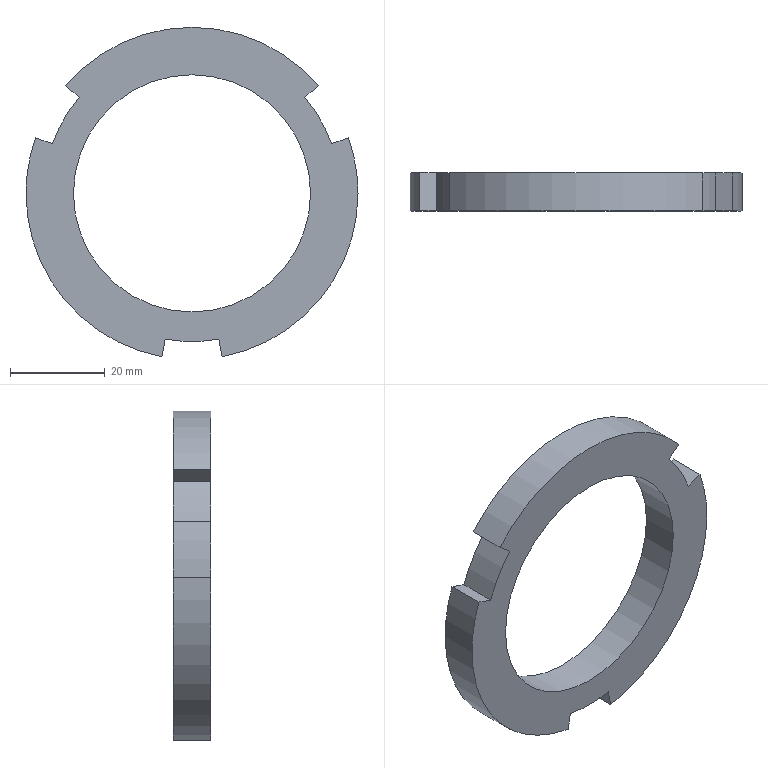Part | STEP file | Input 1-6 | 1 solid | 18 faces | box 70 x 8 x 69.422 mm | volume 13993 mm3 | cylinder 10 | plane 8 | commonest cylinder face diameters 70 x5 62.489 x3 50 x2
STEP:
#1=CARTESIAN_POINT('',(-583.859,1957.264,3172.342));
#2=VERTEX_POINT('',#1);
#3=CARTESIAN_POINT('',(-612.523,1957.264,3137.92));
#4=VERTEX_POINT('',#3);
#5=CARTESIAN_POINT('',(-618.859,1957.264,3172.342));
#6=DIRECTION('',(0.,1.,0.));
#7=DIRECTION('',(1.,0.,0.));
#8=AXIS2_PLACEMENT_3D('',#5,#6,#7);
#9=CIRCLE('',#8,35.);
#10=EDGE_CURVE('',#2,#4,#9,.T.);
#11=ORIENTED_EDGE('',*,*,#10,.F.);
#12=CARTESIAN_POINT('',(-583.859,1949.264,3172.342));
#13=VERTEX_POINT('',#12);
#14=CARTESIAN_POINT('',(-583.859,1957.264,3172.342));
#15=DIRECTION('',(0.,-1.,0.));
#16=VECTOR('',#15,1000.);
#17=LINE('',#14,#16);
#18=EDGE_CURVE('',#2,#13,#17,.T.);
#19=ORIENTED_EDGE('',*,*,#18,.T.);
#20=CARTESIAN_POINT('',(-612.523,1949.264,3137.92));
#21=VERTEX_POINT('',#20);
#22=CARTESIAN_POINT('',(-618.859,1949.264,3172.342));
#23=DIRECTION('',(0.,1.,0.));
#24=DIRECTION('',(1.,0.,0.));
#25=AXIS2_PLACEMENT_3D('',#22,#23,#24);
#26=CIRCLE('',#25,35.);
#27=EDGE_CURVE('',#13,#21,#26,.T.);
#28=ORIENTED_EDGE('',*,*,#27,.T.);
#29=CARTESIAN_POINT('',(-612.523,1957.264,3137.92));
#30=DIRECTION('',(0.,-1.,0.));
#31=VECTOR('',#30,1000.);
#32=LINE('',#29,#31);
#33=EDGE_CURVE('',#4,#21,#32,.T.);
#34=ORIENTED_EDGE('',*,*,#33,.F.);
#35=EDGE_LOOP('',(#11,#19,#28,#34));
#36=FACE_OUTER_BOUND('',#35,.T.);
#37=CARTESIAN_POINT('',(-618.859,1957.264,3172.342));
#38=DIRECTION('',(0.,-1.,0.));
#39=DIRECTION('',(1.,0.,0.));
#40=AXIS2_PLACEMENT_3D('',#37,#38,#39);
#41=CYLINDRICAL_SURFACE('',#40,35.);
#42=ADVANCED_FACE('',(#36),#41,.T.);
#43=CARTESIAN_POINT('',(-643.859,1957.264,3172.342));
#44=VERTEX_POINT('',#43);
#45=CARTESIAN_POINT('',(-593.859,1957.264,3172.342));
#46=VERTEX_POINT('',#45);
#47=CARTESIAN_POINT('',(-618.859,1957.264,3172.342));
#48=DIRECTION('',(0.,1.,0.));
#49=DIRECTION('',(1.,0.,0.));
#50=AXIS2_PLACEMENT_3D('',#47,#48,#49);
#51=CIRCLE('',#50,25.);
#52=EDGE_CURVE('',#44,#46,#51,.T.);
#53=ORIENTED_EDGE('',*,*,#52,.T.);
#54=CARTESIAN_POINT('',(-593.859,1949.264,3172.342));
#55=VERTEX_POINT('',#54);
#56=CARTESIAN_POINT('',(-593.859,1957.264,3172.342));
#57=DIRECTION('',(0.,1.,0.));
#58=VECTOR('',#57,1000.);
#59=LINE('',#56,#58);
#60=EDGE_CURVE('',#55,#46,#59,.T.);
#61=ORIENTED_EDGE('',*,*,#60,.F.);
#62=CARTESIAN_POINT('',(-643.859,1949.264,3172.342));
#63=VERTEX_POINT('',#62);
#64=CARTESIAN_POINT('',(-618.859,1949.264,3172.342));
#65=DIRECTION('',(0.,1.,0.));
#66=DIRECTION('',(1.,0.,0.));
#67=AXIS2_PLACEMENT_3D('',#64,#65,#66);
#68=CIRCLE('',#67,25.);
#69=EDGE_CURVE('',#63,#55,#68,.T.);
#70=ORIENTED_EDGE('',*,*,#69,.F.);
#71=CARTESIAN_POINT('',(-643.859,1957.264,3172.342));
#72=DIRECTION('',(0.,1.,0.));
#73=VECTOR('',#72,1000.);
#74=LINE('',#71,#73);
#75=EDGE_CURVE('',#63,#44,#74,.T.);
#76=ORIENTED_EDGE('',*,*,#75,.T.);
#77=EDGE_LOOP('',(#53,#61,#70,#76));
#78=FACE_OUTER_BOUND('',#77,.T.);
#79=CARTESIAN_POINT('',(-618.859,1957.264,3172.342));
#80=DIRECTION('',(0.,-1.,0.));
#81=DIRECTION('',(1.,0.,0.));
#82=AXIS2_PLACEMENT_3D('',#79,#80,#81);
#83=CYLINDRICAL_SURFACE('',#82,25.);
#84=ADVANCED_FACE('',(#78),#83,.F.);
#85=CARTESIAN_POINT('',(-653.859,1957.264,3172.342));
#86=VERTEX_POINT('',#85);
#87=CARTESIAN_POINT('',(-651.837,1957.264,3184.066));
#88=VERTEX_POINT('',#87);
#89=CARTESIAN_POINT('',(-618.859,1957.264,3172.342));
#90=DIRECTION('',(0.,1.,0.));
#91=DIRECTION('',(1.,0.,0.));
#92=AXIS2_PLACEMENT_3D('',#89,#90,#91);
#93=CIRCLE('',#92,35.);
#94=EDGE_CURVE('',#86,#88,#93,.T.);
#95=ORIENTED_EDGE('',*,*,#94,.F.);
#96=CARTESIAN_POINT('',(-653.859,1949.264,3172.342));
#97=VERTEX_POINT('',#96);
#98=CARTESIAN_POINT('',(-653.859,1957.264,3172.342));
#99=DIRECTION('',(0.,-1.,0.));
#100=VECTOR('',#99,1000.);
#101=LINE('',#98,#100);
#102=EDGE_CURVE('',#86,#97,#101,.T.);
#103=ORIENTED_EDGE('',*,*,#102,.T.);
#104=CARTESIAN_POINT('',(-651.837,1949.264,3184.066));
#105=VERTEX_POINT('',#104);
#106=CARTESIAN_POINT('',(-618.859,1949.264,3172.342));
#107=DIRECTION('',(0.,1.,0.));
#108=DIRECTION('',(1.,0.,0.));
#109=AXIS2_PLACEMENT_3D('',#106,#107,#108);
#110=CIRCLE('',#109,35.);
#111=EDGE_CURVE('',#97,#105,#110,.T.);
#112=ORIENTED_EDGE('',*,*,#111,.T.);
#113=CARTESIAN_POINT('',(-651.837,1957.264,3184.066));
#114=DIRECTION('',(0.,-1.,0.));
#115=VECTOR('',#114,1000.);
#116=LINE('',#113,#115);
#117=EDGE_CURVE('',#88,#105,#116,.T.);
#118=ORIENTED_EDGE('',*,*,#117,.F.);
#119=EDGE_LOOP('',(#95,#103,#112,#118));
#120=FACE_OUTER_BOUND('',#119,.T.);
#121=CARTESIAN_POINT('',(-618.859,1957.264,3172.342));
#122=DIRECTION('',(0.,-1.,0.));
#123=DIRECTION('',(1.,0.,0.));
#124=AXIS2_PLACEMENT_3D('',#121,#122,#123);
#125=CYLINDRICAL_SURFACE('',#124,35.);
#126=ADVANCED_FACE('',(#120),#125,.T.);
#127=CARTESIAN_POINT('',(-613.203,1957.264,3141.613));
#128=VERTEX_POINT('',#127);
#129=CARTESIAN_POINT('',(-624.515,1957.264,3141.613));
#130=VERTEX_POINT('',#129);
#131=CARTESIAN_POINT('',(-618.859,1957.264,3172.342));
#132=DIRECTION('',(0.,1.,0.));
#133=DIRECTION('',(1.,0.,0.));
#134=AXIS2_PLACEMENT_3D('',#131,#132,#133);
#135=CIRCLE('',#134,31.244);
#136=EDGE_CURVE('',#128,#130,#135,.T.);
#137=ORIENTED_EDGE('',*,*,#136,.T.);
#138=CARTESIAN_POINT('',(-625.195,1957.264,3137.92));
#139=VERTEX_POINT('',#138);
#140=CARTESIAN_POINT('',(-625.195,1957.264,3137.92));
#141=DIRECTION('',(-0.181,0.,-0.9835));
#142=VECTOR('',#141,1000.);
#143=LINE('',#140,#142);
#144=EDGE_CURVE('',#130,#139,#143,.T.);
#145=ORIENTED_EDGE('',*,*,#144,.T.);
#146=CARTESIAN_POINT('',(-618.859,1957.264,3172.342));
#147=DIRECTION('',(0.,1.,0.));
#148=DIRECTION('',(1.,0.,0.));
#149=AXIS2_PLACEMENT_3D('',#146,#147,#148);
#150=CIRCLE('',#149,35.);
#151=EDGE_CURVE('',#139,#86,#150,.T.);
#152=ORIENTED_EDGE('',*,*,#151,.T.);
#153=ORIENTED_EDGE('',*,*,#94,.T.);
#154=CARTESIAN_POINT('',(-648.298,1957.264,3182.808));
#155=VERTEX_POINT('',#154);
#156=CARTESIAN_POINT('',(-651.837,1957.264,3184.066));
#157=DIRECTION('',(0.9422,0.,-0.335));
#158=VECTOR('',#157,1000.);
#159=LINE('',#156,#158);
#160=EDGE_CURVE('',#88,#155,#159,.T.);
#161=ORIENTED_EDGE('',*,*,#160,.T.);
#162=CARTESIAN_POINT('',(-642.642,1957.264,3192.604));
#163=VERTEX_POINT('',#162);
#164=CARTESIAN_POINT('',(-618.859,1957.264,3172.342));
#165=DIRECTION('',(0.,1.,0.));
#166=DIRECTION('',(1.,0.,0.));
#167=AXIS2_PLACEMENT_3D('',#164,#165,#166);
#168=CIRCLE('',#167,31.244);
#169=EDGE_CURVE('',#155,#163,#168,.T.);
#170=ORIENTED_EDGE('',*,*,#169,.T.);
#171=CARTESIAN_POINT('',(-645.501,1957.264,3195.04));
#172=VERTEX_POINT('',#171);
#173=CARTESIAN_POINT('',(-645.501,1957.264,3195.04));
#174=DIRECTION('',(-0.7612,0.,0.6485));
#175=VECTOR('',#174,1000.);
#176=LINE('',#173,#175);
#177=EDGE_CURVE('',#163,#172,#176,.T.);
#178=ORIENTED_EDGE('',*,*,#177,.T.);
#179=CARTESIAN_POINT('',(-592.217,1957.264,3195.04));
#180=VERTEX_POINT('',#179);
#181=CARTESIAN_POINT('',(-618.859,1957.264,3172.342));
#182=DIRECTION('',(0.,1.,0.));
#183=DIRECTION('',(1.,0.,0.));
#184=AXIS2_PLACEMENT_3D('',#181,#182,#183);
#185=CIRCLE('',#184,35.);
#186=EDGE_CURVE('',#172,#180,#185,.T.);
#187=ORIENTED_EDGE('',*,*,#186,.T.);
#188=CARTESIAN_POINT('',(-595.075,1957.264,3192.604));
#189=VERTEX_POINT('',#188);
#190=CARTESIAN_POINT('',(-592.217,1957.264,3195.04));
#191=DIRECTION('',(-0.7612,0.,-0.6485));
#192=VECTOR('',#191,1000.);
#193=LINE('',#190,#192);
#194=EDGE_CURVE('',#180,#189,#193,.T.);
#195=ORIENTED_EDGE('',*,*,#194,.T.);
#196=CARTESIAN_POINT('',(-589.419,1957.264,3182.808));
#197=VERTEX_POINT('',#196);
#198=CARTESIAN_POINT('',(-618.859,1957.264,3172.342));
#199=DIRECTION('',(0.,1.,0.));
#200=DIRECTION('',(1.,0.,0.));
#201=AXIS2_PLACEMENT_3D('',#198,#199,#200);
#202=CIRCLE('',#201,31.244);
#203=EDGE_CURVE('',#189,#197,#202,.T.);
#204=ORIENTED_EDGE('',*,*,#203,.T.);
#205=CARTESIAN_POINT('',(-585.881,1957.264,3184.066));
#206=VERTEX_POINT('',#205);
#207=CARTESIAN_POINT('',(-585.881,1957.264,3184.066));
#208=DIRECTION('',(0.9422,0.,0.335));
#209=VECTOR('',#208,1000.);
#210=LINE('',#207,#209);
#211=EDGE_CURVE('',#197,#206,#210,.T.);
#212=ORIENTED_EDGE('',*,*,#211,.T.);
#213=CARTESIAN_POINT('',(-618.859,1957.264,3172.342));
#214=DIRECTION('',(0.,1.,0.));
#215=DIRECTION('',(1.,0.,0.));
#216=AXIS2_PLACEMENT_3D('',#213,#214,#215);
#217=CIRCLE('',#216,35.);
#218=EDGE_CURVE('',#206,#2,#217,.T.);
#219=ORIENTED_EDGE('',*,*,#218,.T.);
#220=ORIENTED_EDGE('',*,*,#10,.T.);
#221=CARTESIAN_POINT('',(-612.523,1957.264,3137.92));
#222=DIRECTION('',(-0.181,0.,0.9835));
#223=VECTOR('',#222,1000.);
#224=LINE('',#221,#223);
#225=EDGE_CURVE('',#4,#128,#224,.T.);
#226=ORIENTED_EDGE('',*,*,#225,.T.);
#227=EDGE_LOOP('',(#137,#145,#152,#153,#161,#170,#178,#187,#195,#204,#212,#219,#220,#226));
#228=FACE_OUTER_BOUND('',#227,.T.);
#229=ORIENTED_EDGE('',*,*,#52,.F.);
#230=CARTESIAN_POINT('',(-618.859,1957.264,3172.342));
#231=DIRECTION('',(0.,1.,0.));
#232=DIRECTION('',(1.,0.,0.));
#233=AXIS2_PLACEMENT_3D('',#230,#231,#232);
#234=CIRCLE('',#233,25.);
#235=EDGE_CURVE('',#46,#44,#234,.T.);
#236=ORIENTED_EDGE('',*,*,#235,.F.);
#237=EDGE_LOOP('',(#229,#236));
#238=FACE_BOUND('',#237,.T.);
#239=CARTESIAN_POINT('',(-618.859,1957.264,3172.342));
#240=DIRECTION('',(0.,1.,0.));
#241=DIRECTION('',(-1.,0.,0.));
#242=AXIS2_PLACEMENT_3D('',#239,#240,#241);
#243=PLANE('',#242);
#244=ADVANCED_FACE('',(#228,#238),#243,.T.);
#245=CARTESIAN_POINT('',(-613.203,1949.264,3141.613));
#246=VERTEX_POINT('',#245);
#247=CARTESIAN_POINT('',(-624.515,1949.264,3141.613));
#248=VERTEX_POINT('',#247);
#249=CARTESIAN_POINT('',(-618.859,1949.264,3172.342));
#250=DIRECTION('',(0.,1.,0.));
#251=DIRECTION('',(1.,0.,0.));
#252=AXIS2_PLACEMENT_3D('',#249,#250,#251);
#253=CIRCLE('',#252,31.244);
#254=EDGE_CURVE('',#246,#248,#253,.T.);
#255=ORIENTED_EDGE('',*,*,#254,.F.);
#256=CARTESIAN_POINT('',(-612.523,1949.264,3137.92));
#257=DIRECTION('',(-0.181,0.,0.9835));
#258=VECTOR('',#257,1000.);
#259=LINE('',#256,#258);
#260=EDGE_CURVE('',#21,#246,#259,.T.);
#261=ORIENTED_EDGE('',*,*,#260,.F.);
#262=ORIENTED_EDGE('',*,*,#27,.F.);
#263=CARTESIAN_POINT('',(-585.881,1949.264,3184.066));
#264=VERTEX_POINT('',#263);
#265=CARTESIAN_POINT('',(-618.859,1949.264,3172.342));
#266=DIRECTION('',(0.,1.,0.));
#267=DIRECTION('',(1.,0.,0.));
#268=AXIS2_PLACEMENT_3D('',#265,#266,#267);
#269=CIRCLE('',#268,35.);
#270=EDGE_CURVE('',#264,#13,#269,.T.);
#271=ORIENTED_EDGE('',*,*,#270,.F.);
#272=CARTESIAN_POINT('',(-589.419,1949.264,3182.808));
#273=VERTEX_POINT('',#272);
#274=CARTESIAN_POINT('',(-585.881,1949.264,3184.066));
#275=DIRECTION('',(0.9422,0.,0.335));
#276=VECTOR('',#275,1000.);
#277=LINE('',#274,#276);
#278=EDGE_CURVE('',#273,#264,#277,.T.);
#279=ORIENTED_EDGE('',*,*,#278,.F.);
#280=CARTESIAN_POINT('',(-595.075,1949.264,3192.604));
#281=VERTEX_POINT('',#280);
#282=CARTESIAN_POINT('',(-618.859,1949.264,3172.342));
#283=DIRECTION('',(0.,1.,0.));
#284=DIRECTION('',(1.,0.,0.));
#285=AXIS2_PLACEMENT_3D('',#282,#283,#284);
#286=CIRCLE('',#285,31.244);
#287=EDGE_CURVE('',#281,#273,#286,.T.);
#288=ORIENTED_EDGE('',*,*,#287,.F.);
#289=CARTESIAN_POINT('',(-592.217,1949.264,3195.04));
#290=VERTEX_POINT('',#289);
#291=CARTESIAN_POINT('',(-592.217,1949.264,3195.04));
#292=DIRECTION('',(-0.7612,0.,-0.6485));
#293=VECTOR('',#292,1000.);
#294=LINE('',#291,#293);
#295=EDGE_CURVE('',#290,#281,#294,.T.);
#296=ORIENTED_EDGE('',*,*,#295,.F.);
#297=CARTESIAN_POINT('',(-645.501,1949.264,3195.04));
#298=VERTEX_POINT('',#297);
#299=CARTESIAN_POINT('',(-618.859,1949.264,3172.342));
#300=DIRECTION('',(0.,1.,0.));
#301=DIRECTION('',(1.,0.,0.));
#302=AXIS2_PLACEMENT_3D('',#299,#300,#301);
#303=CIRCLE('',#302,35.);
#304=EDGE_CURVE('',#298,#290,#303,.T.);
#305=ORIENTED_EDGE('',*,*,#304,.F.);
#306=CARTESIAN_POINT('',(-642.642,1949.264,3192.604));
#307=VERTEX_POINT('',#306);
#308=CARTESIAN_POINT('',(-645.501,1949.264,3195.04));
#309=DIRECTION('',(-0.7612,0.,0.6485));
#310=VECTOR('',#309,1000.);
#311=LINE('',#308,#310);
#312=EDGE_CURVE('',#307,#298,#311,.T.);
#313=ORIENTED_EDGE('',*,*,#312,.F.);
#314=CARTESIAN_POINT('',(-648.298,1949.264,3182.808));
#315=VERTEX_POINT('',#314);
#316=CARTESIAN_POINT('',(-618.859,1949.264,3172.342));
#317=DIRECTION('',(0.,1.,0.));
#318=DIRECTION('',(1.,0.,0.));
#319=AXIS2_PLACEMENT_3D('',#316,#317,#318);
#320=CIRCLE('',#319,31.244);
#321=EDGE_CURVE('',#315,#307,#320,.T.);
#322=ORIENTED_EDGE('',*,*,#321,.F.);
#323=CARTESIAN_POINT('',(-651.837,1949.264,3184.066));
#324=DIRECTION('',(0.9422,0.,-0.335));
#325=VECTOR('',#324,1000.);
#326=LINE('',#323,#325);
#327=EDGE_CURVE('',#105,#315,#326,.T.);
#328=ORIENTED_EDGE('',*,*,#327,.F.);
#329=ORIENTED_EDGE('',*,*,#111,.F.);
#330=CARTESIAN_POINT('',(-625.195,1949.264,3137.92));
#331=VERTEX_POINT('',#330);
#332=CARTESIAN_POINT('',(-618.859,1949.264,3172.342));
#333=DIRECTION('',(0.,1.,0.));
#334=DIRECTION('',(1.,0.,0.));
#335=AXIS2_PLACEMENT_3D('',#332,#333,#334);
#336=CIRCLE('',#335,35.);
#337=EDGE_CURVE('',#331,#97,#336,.T.);
#338=ORIENTED_EDGE('',*,*,#337,.F.);
#339=CARTESIAN_POINT('',(-625.195,1949.264,3137.92));
#340=DIRECTION('',(-0.181,0.,-0.9835));
#341=VECTOR('',#340,1000.);
#342=LINE('',#339,#341);
#343=EDGE_CURVE('',#248,#331,#342,.T.);
#344=ORIENTED_EDGE('',*,*,#343,.F.);
#345=EDGE_LOOP('',(#255,#261,#262,#271,#279,#288,#296,#305,#313,#322,#328,#329,#338,#344));
#346=FACE_OUTER_BOUND('',#345,.T.);
#347=ORIENTED_EDGE('',*,*,#69,.T.);
#348=CARTESIAN_POINT('',(-618.859,1949.264,3172.342));
#349=DIRECTION('',(0.,1.,0.));
#350=DIRECTION('',(1.,0.,0.));
#351=AXIS2_PLACEMENT_3D('',#348,#349,#350);
#352=CIRCLE('',#351,25.);
#353=EDGE_CURVE('',#55,#63,#352,.T.);
#354=ORIENTED_EDGE('',*,*,#353,.T.);
#355=EDGE_LOOP('',(#347,#354));
#356=FACE_BOUND('',#355,.T.);
#357=CARTESIAN_POINT('',(-618.859,1949.264,3172.342));
#358=DIRECTION('',(0.,1.,0.));
#359=DIRECTION('',(-1.,0.,0.));
#360=AXIS2_PLACEMENT_3D('',#357,#358,#359);
#361=PLANE('',#360);
#362=ADVANCED_FACE('',(#346,#356),#361,.F.);
#363=ORIENTED_EDGE('',*,*,#254,.T.);
#364=CARTESIAN_POINT('',(-624.515,1957.264,3141.613));
#365=DIRECTION('',(0.,-1.,0.));
#366=VECTOR('',#365,1000.);
#367=LINE('',#364,#366);
#368=EDGE_CURVE('',#130,#248,#367,.T.);
#369=ORIENTED_EDGE('',*,*,#368,.F.);
#370=ORIENTED_EDGE('',*,*,#136,.F.);
#371=CARTESIAN_POINT('',(-613.203,1957.264,3141.613));
#372=DIRECTION('',(0.,-1.,0.));
#373=VECTOR('',#372,1000.);
#374=LINE('',#371,#373);
#375=EDGE_CURVE('',#128,#246,#374,.T.);
#376=ORIENTED_EDGE('',*,*,#375,.T.);
#377=EDGE_LOOP('',(#363,#369,#370,#376));
#378=FACE_OUTER_BOUND('',#377,.T.);
#379=CARTESIAN_POINT('',(-618.859,1957.264,3172.342));
#380=DIRECTION('',(0.,-1.,0.));
#381=DIRECTION('',(1.,0.,0.));
#382=AXIS2_PLACEMENT_3D('',#379,#380,#381);
#383=CYLINDRICAL_SURFACE('',#382,31.244);
#384=ADVANCED_FACE('',(#378),#383,.T.);
#385=ORIENTED_EDGE('',*,*,#343,.T.);
#386=CARTESIAN_POINT('',(-625.195,1957.264,3137.92));
#387=DIRECTION('',(0.,-1.,0.));
#388=VECTOR('',#387,1000.);
#389=LINE('',#386,#388);
#390=EDGE_CURVE('',#139,#331,#389,.T.);
#391=ORIENTED_EDGE('',*,*,#390,.F.);
#392=ORIENTED_EDGE('',*,*,#144,.F.);
#393=ORIENTED_EDGE('',*,*,#368,.T.);
#394=EDGE_LOOP('',(#385,#391,#392,#393));
#395=FACE_OUTER_BOUND('',#394,.T.);
#396=CARTESIAN_POINT('',(-625.195,1957.264,3137.92));
#397=DIRECTION('',(-0.9835,0.,0.181));
#398=DIRECTION('',(-0.181,0.,-0.9835));
#399=AXIS2_PLACEMENT_3D('',#396,#397,#398);
#400=PLANE('',#399);
#401=ADVANCED_FACE('',(#395),#400,.F.);
#402=ORIENTED_EDGE('',*,*,#102,.F.);
#403=ORIENTED_EDGE('',*,*,#151,.F.);
#404=ORIENTED_EDGE('',*,*,#390,.T.);
#405=ORIENTED_EDGE('',*,*,#337,.T.);
#406=EDGE_LOOP('',(#402,#403,#404,#405));
#407=FACE_OUTER_BOUND('',#406,.T.);
#408=CARTESIAN_POINT('',(-618.859,1957.264,3172.342));
#409=DIRECTION('',(0.,-1.,0.));
#410=DIRECTION('',(1.,0.,0.));
#411=AXIS2_PLACEMENT_3D('',#408,#409,#410);
#412=CYLINDRICAL_SURFACE('',#411,35.);
#413=ADVANCED_FACE('',(#407),#412,.T.);
#414=ORIENTED_EDGE('',*,*,#327,.T.);
#415=CARTESIAN_POINT('',(-648.298,1957.264,3182.808));
#416=DIRECTION('',(0.,-1.,0.));
#417=VECTOR('',#416,1000.);
#418=LINE('',#415,#417);
#419=EDGE_CURVE('',#155,#315,#418,.T.);
#420=ORIENTED_EDGE('',*,*,#419,.F.);
#421=ORIENTED_EDGE('',*,*,#160,.F.);
#422=ORIENTED_EDGE('',*,*,#117,.T.);
#423=EDGE_LOOP('',(#414,#420,#421,#422));
#424=FACE_OUTER_BOUND('',#423,.T.);
#425=CARTESIAN_POINT('',(-651.837,1957.264,3184.066));
#426=DIRECTION('',(-0.335,0.,-0.9422));
#427=DIRECTION('',(0.9422,0.,-0.335));
#428=AXIS2_PLACEMENT_3D('',#425,#426,#427);
#429=PLANE('',#428);
#430=ADVANCED_FACE('',(#424),#429,.F.);
#431=ORIENTED_EDGE('',*,*,#321,.T.);
#432=CARTESIAN_POINT('',(-642.642,1957.264,3192.604));
#433=DIRECTION('',(0.,-1.,0.));
#434=VECTOR('',#433,1000.);
#435=LINE('',#432,#434);
#436=EDGE_CURVE('',#163,#307,#435,.T.);
#437=ORIENTED_EDGE('',*,*,#436,.F.);
#438=ORIENTED_EDGE('',*,*,#169,.F.);
#439=ORIENTED_EDGE('',*,*,#419,.T.);
#440=EDGE_LOOP('',(#431,#437,#438,#439));
#441=FACE_OUTER_BOUND('',#440,.T.);
#442=CARTESIAN_POINT('',(-618.859,1957.264,3172.342));
#443=DIRECTION('',(0.,-1.,0.));
#444=DIRECTION('',(1.,0.,0.));
#445=AXIS2_PLACEMENT_3D('',#442,#443,#444);
#446=CYLINDRICAL_SURFACE('',#445,31.244);
#447=ADVANCED_FACE('',(#441),#446,.T.);
#448=ORIENTED_EDGE('',*,*,#312,.T.);
#449=CARTESIAN_POINT('',(-645.501,1957.264,3195.04));
#450=DIRECTION('',(0.,-1.,0.));
#451=VECTOR('',#450,1000.);
#452=LINE('',#449,#451);
#453=EDGE_CURVE('',#172,#298,#452,.T.);
#454=ORIENTED_EDGE('',*,*,#453,.F.);
#455=ORIENTED_EDGE('',*,*,#177,.F.);
#456=ORIENTED_EDGE('',*,*,#436,.T.);
#457=EDGE_LOOP('',(#448,#454,#455,#456));
#458=FACE_OUTER_BOUND('',#457,.T.);
#459=CARTESIAN_POINT('',(-645.501,1957.264,3195.04));
#460=DIRECTION('',(0.6485,0.,0.7612));
#461=DIRECTION('',(-0.7612,0.,0.6485));
#462=AXIS2_PLACEMENT_3D('',#459,#460,#461);
#463=PLANE('',#462);
#464=ADVANCED_FACE('',(#458),#463,.F.);
#465=ORIENTED_EDGE('',*,*,#304,.T.);
#466=CARTESIAN_POINT('',(-592.217,1957.264,3195.04));
#467=DIRECTION('',(0.,-1.,0.));
#468=VECTOR('',#467,1000.);
#469=LINE('',#466,#468);
#470=EDGE_CURVE('',#180,#290,#469,.T.);
#471=ORIENTED_EDGE('',*,*,#470,.F.);
#472=ORIENTED_EDGE('',*,*,#186,.F.);
#473=ORIENTED_EDGE('',*,*,#453,.T.);
#474=EDGE_LOOP('',(#465,#471,#472,#473));
#475=FACE_OUTER_BOUND('',#474,.T.);
#476=CARTESIAN_POINT('',(-618.859,1957.264,3172.342));
#477=DIRECTION('',(0.,-1.,0.));
#478=DIRECTION('',(1.,0.,0.));
#479=AXIS2_PLACEMENT_3D('',#476,#477,#478);
#480=CYLINDRICAL_SURFACE('',#479,35.);
#481=ADVANCED_FACE('',(#475),#480,.T.);
#482=ORIENTED_EDGE('',*,*,#295,.T.);
#483=CARTESIAN_POINT('',(-595.075,1957.264,3192.604));
#484=DIRECTION('',(0.,-1.,0.));
#485=VECTOR('',#484,1000.);
#486=LINE('',#483,#485);
#487=EDGE_CURVE('',#189,#281,#486,.T.);
#488=ORIENTED_EDGE('',*,*,#487,.F.);
#489=ORIENTED_EDGE('',*,*,#194,.F.);
#490=ORIENTED_EDGE('',*,*,#470,.T.);
#491=EDGE_LOOP('',(#482,#488,#489,#490));
#492=FACE_OUTER_BOUND('',#491,.T.);
#493=CARTESIAN_POINT('',(-592.217,1957.264,3195.04));
#494=DIRECTION('',(-0.6485,0.,0.7612));
#495=DIRECTION('',(-0.7612,0.,-0.6485));
#496=AXIS2_PLACEMENT_3D('',#493,#494,#495);
#497=PLANE('',#496);
#498=ADVANCED_FACE('',(#492),#497,.F.);
#499=ORIENTED_EDGE('',*,*,#287,.T.);
#500=CARTESIAN_POINT('',(-589.419,1957.264,3182.808));
#501=DIRECTION('',(0.,-1.,0.));
#502=VECTOR('',#501,1000.);
#503=LINE('',#500,#502);
#504=EDGE_CURVE('',#197,#273,#503,.T.);
#505=ORIENTED_EDGE('',*,*,#504,.F.);
#506=ORIENTED_EDGE('',*,*,#203,.F.);
#507=ORIENTED_EDGE('',*,*,#487,.T.);
#508=EDGE_LOOP('',(#499,#505,#506,#507));
#509=FACE_OUTER_BOUND('',#508,.T.);
#510=CARTESIAN_POINT('',(-618.859,1957.264,3172.342));
#511=DIRECTION('',(0.,-1.,0.));
#512=DIRECTION('',(1.,0.,0.));
#513=AXIS2_PLACEMENT_3D('',#510,#511,#512);
#514=CYLINDRICAL_SURFACE('',#513,31.244);
#515=ADVANCED_FACE('',(#509),#514,.T.);
#516=ORIENTED_EDGE('',*,*,#278,.T.);
#517=CARTESIAN_POINT('',(-585.881,1957.264,3184.066));
#518=DIRECTION('',(0.,-1.,0.));
#519=VECTOR('',#518,1000.);
#520=LINE('',#517,#519);
#521=EDGE_CURVE('',#206,#264,#520,.T.);
#522=ORIENTED_EDGE('',*,*,#521,.F.);
#523=ORIENTED_EDGE('',*,*,#211,.F.);
#524=ORIENTED_EDGE('',*,*,#504,.T.);
#525=EDGE_LOOP('',(#516,#522,#523,#524));
#526=FACE_OUTER_BOUND('',#525,.T.);
#527=CARTESIAN_POINT('',(-585.881,1957.264,3184.066));
#528=DIRECTION('',(0.335,0.,-0.9422));
#529=DIRECTION('',(0.9422,0.,0.335));
#530=AXIS2_PLACEMENT_3D('',#527,#528,#529);
#531=PLANE('',#530);
#532=ADVANCED_FACE('',(#526),#531,.F.);
#533=ORIENTED_EDGE('',*,*,#18,.F.);
#534=ORIENTED_EDGE('',*,*,#218,.F.);
#535=ORIENTED_EDGE('',*,*,#521,.T.);
#536=ORIENTED_EDGE('',*,*,#270,.T.);
#537=EDGE_LOOP('',(#533,#534,#535,#536));
#538=FACE_OUTER_BOUND('',#537,.T.);
#539=CARTESIAN_POINT('',(-618.859,1957.264,3172.342));
#540=DIRECTION('',(0.,-1.,0.));
#541=DIRECTION('',(1.,0.,0.));
#542=AXIS2_PLACEMENT_3D('',#539,#540,#541);
#543=CYLINDRICAL_SURFACE('',#542,35.);
#544=ADVANCED_FACE('',(#538),#543,.T.);
#545=ORIENTED_EDGE('',*,*,#260,.T.);
#546=ORIENTED_EDGE('',*,*,#375,.F.);
#547=ORIENTED_EDGE('',*,*,#225,.F.);
#548=ORIENTED_EDGE('',*,*,#33,.T.);
#549=EDGE_LOOP('',(#545,#546,#547,#548));
#550=FACE_OUTER_BOUND('',#549,.T.);
#551=CARTESIAN_POINT('',(-612.523,1957.264,3137.92));
#552=DIRECTION('',(0.9835,0.,0.181));
#553=DIRECTION('',(-0.181,0.,0.9835));
#554=AXIS2_PLACEMENT_3D('',#551,#552,#553);
#555=PLANE('',#554);
#556=ADVANCED_FACE('',(#550),#555,.F.);
#557=ORIENTED_EDGE('',*,*,#60,.T.);
#558=ORIENTED_EDGE('',*,*,#235,.T.);
#559=ORIENTED_EDGE('',*,*,#75,.F.);
#560=ORIENTED_EDGE('',*,*,#353,.F.);
#561=EDGE_LOOP('',(#557,#558,#559,#560));
#562=FACE_OUTER_BOUND('',#561,.T.);
#563=CARTESIAN_POINT('',(-618.859,1957.264,3172.342));
#564=DIRECTION('',(0.,-1.,0.));
#565=DIRECTION('',(1.,0.,0.));
#566=AXIS2_PLACEMENT_3D('',#563,#564,#565);
#567=CYLINDRICAL_SURFACE('',#566,25.);
#568=ADVANCED_FACE('',(#562),#567,.F.);
#569=CLOSED_SHELL('',(#42,#84,#126,#244,#362,#384,#401,#413,#430,#447,#464,#481,#498,#515,#532,#544,#556,#568));
#570=MANIFOLD_SOLID_BREP('',#569);
#571=CARTESIAN_POINT('',(0.,0.,0.));
#572=DIRECTION('',(0.,0.,1.));
#573=DIRECTION('',(1.,0.,0.));
#574=AXIS2_PLACEMENT_3D('',#571,#572,#573);
#575=(LENGTH_UNIT()NAMED_UNIT(*)SI_UNIT(.MILLI.,.METRE.));
#576=UNCERTAINTY_MEASURE_WITH_UNIT(LENGTH_MEASURE(0.00001),#575,'','');
#577=(NAMED_UNIT(*)PLANE_ANGLE_UNIT()SI_UNIT($,.RADIAN.));
#578=(NAMED_UNIT(*)SI_UNIT($,.STERADIAN.)SOLID_ANGLE_UNIT());
#579=(GEOMETRIC_REPRESENTATION_CONTEXT(3)GLOBAL_UNCERTAINTY_ASSIGNED_CONTEXT((#576))GLOBAL_UNIT_ASSIGNED_CONTEXT((#575,#577,#578))REPRESENTATION_CONTEXT('',''));
#580=ADVANCED_BREP_SHAPE_REPRESENTATION('',(#570,#574),#579);